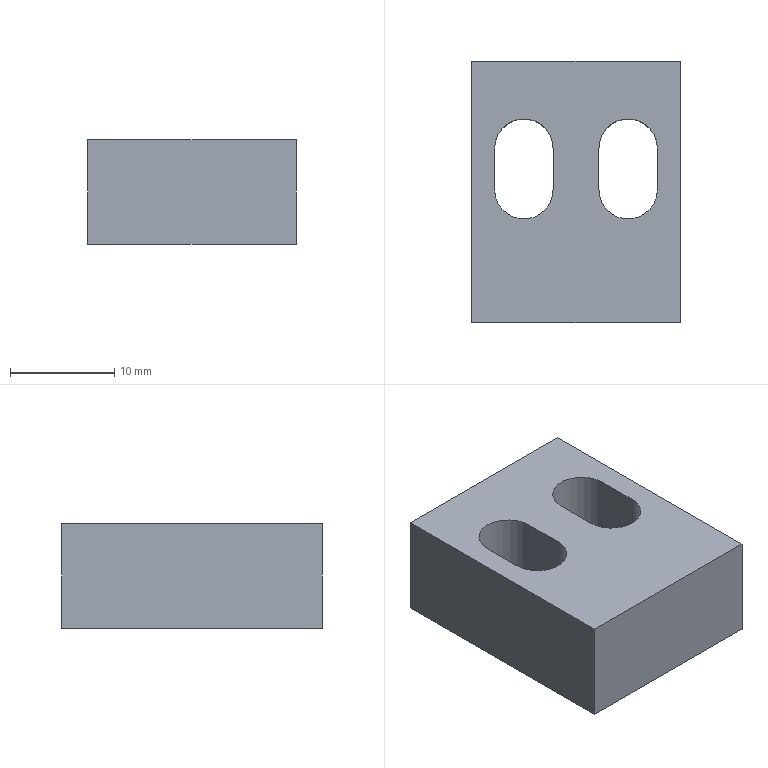Part | 1 solid | 14 faces | box 20 x 25 x 10 mm | volume 4059 mm3 | plane 10 | cylinder 4 | commonest cylinder face diameters 5.6 x4
STEP:
#1=CARTESIAN_POINT('',(-7.8,0.2,10.));
#2=VERTEX_POINT('',#1);
#3=CARTESIAN_POINT('',(-2.2,0.2,10.));
#4=VERTEX_POINT('',#3);
#5=CARTESIAN_POINT('',(-5.,0.2,10.));
#6=DIRECTION('',(0.,0.,1.));
#7=DIRECTION('',(1.,0.,0.));
#8=AXIS2_PLACEMENT_3D('',#5,#6,#7);
#9=CIRCLE('',#8,2.8);
#10=EDGE_CURVE('',#2,#4,#9,.T.);
#11=ORIENTED_EDGE('',*,*,#10,.F.);
#12=CARTESIAN_POINT('',(-7.8,4.2,10.));
#13=VERTEX_POINT('',#12);
#14=CARTESIAN_POINT('',(-7.8,0.2,10.));
#15=DIRECTION('',(0.,-1.,0.));
#16=VECTOR('',#15,1000.);
#17=LINE('',#14,#16);
#18=EDGE_CURVE('',#13,#2,#17,.T.);
#19=ORIENTED_EDGE('',*,*,#18,.F.);
#20=CARTESIAN_POINT('',(-2.2,4.2,10.));
#21=VERTEX_POINT('',#20);
#22=CARTESIAN_POINT('',(-5.,4.2,10.));
#23=DIRECTION('',(0.,0.,1.));
#24=DIRECTION('',(1.,0.,0.));
#25=AXIS2_PLACEMENT_3D('',#22,#23,#24);
#26=CIRCLE('',#25,2.8);
#27=EDGE_CURVE('',#21,#13,#26,.T.);
#28=ORIENTED_EDGE('',*,*,#27,.F.);
#29=CARTESIAN_POINT('',(-2.2,0.2,10.));
#30=DIRECTION('',(0.,1.,0.));
#31=VECTOR('',#30,1000.);
#32=LINE('',#29,#31);
#33=EDGE_CURVE('',#4,#21,#32,.T.);
#34=ORIENTED_EDGE('',*,*,#33,.F.);
#35=EDGE_LOOP('',(#11,#19,#28,#34));
#36=FACE_BOUND('',#35,.T.);
#37=CARTESIAN_POINT('',(10.,-12.5,10.));
#38=VERTEX_POINT('',#37);
#39=CARTESIAN_POINT('',(10.,12.5,10.));
#40=VERTEX_POINT('',#39);
#41=CARTESIAN_POINT('',(10.,-12.5,10.));
#42=DIRECTION('',(0.,1.,0.));
#43=VECTOR('',#42,1000.);
#44=LINE('',#41,#43);
#45=EDGE_CURVE('',#38,#40,#44,.T.);
#46=ORIENTED_EDGE('',*,*,#45,.T.);
#47=CARTESIAN_POINT('',(-10.,12.5,10.));
#48=VERTEX_POINT('',#47);
#49=CARTESIAN_POINT('',(-10.,12.5,10.));
#50=DIRECTION('',(-1.,0.,0.));
#51=VECTOR('',#50,1000.);
#52=LINE('',#49,#51);
#53=EDGE_CURVE('',#40,#48,#52,.T.);
#54=ORIENTED_EDGE('',*,*,#53,.T.);
#55=CARTESIAN_POINT('',(-10.,-12.5,10.));
#56=VERTEX_POINT('',#55);
#57=CARTESIAN_POINT('',(-10.,-12.5,10.));
#58=DIRECTION('',(0.,-1.,0.));
#59=VECTOR('',#58,1000.);
#60=LINE('',#57,#59);
#61=EDGE_CURVE('',#48,#56,#60,.T.);
#62=ORIENTED_EDGE('',*,*,#61,.T.);
#63=CARTESIAN_POINT('',(-10.,-12.5,10.));
#64=DIRECTION('',(1.,0.,0.));
#65=VECTOR('',#64,1000.);
#66=LINE('',#63,#65);
#67=EDGE_CURVE('',#56,#38,#66,.T.);
#68=ORIENTED_EDGE('',*,*,#67,.T.);
#69=EDGE_LOOP('',(#46,#54,#62,#68));
#70=FACE_OUTER_BOUND('',#69,.T.);
#71=CARTESIAN_POINT('',(2.2,0.2,10.));
#72=VERTEX_POINT('',#71);
#73=CARTESIAN_POINT('',(7.8,0.2,10.));
#74=VERTEX_POINT('',#73);
#75=CARTESIAN_POINT('',(5.,0.2,10.));
#76=DIRECTION('',(0.,0.,1.));
#77=DIRECTION('',(-1.,0.,0.));
#78=AXIS2_PLACEMENT_3D('',#75,#76,#77);
#79=CIRCLE('',#78,2.8);
#80=EDGE_CURVE('',#72,#74,#79,.T.);
#81=ORIENTED_EDGE('',*,*,#80,.F.);
#82=CARTESIAN_POINT('',(2.2,4.2,10.));
#83=VERTEX_POINT('',#82);
#84=CARTESIAN_POINT('',(2.2,0.2,10.));
#85=DIRECTION('',(0.,-1.,0.));
#86=VECTOR('',#85,1000.);
#87=LINE('',#84,#86);
#88=EDGE_CURVE('',#83,#72,#87,.T.);
#89=ORIENTED_EDGE('',*,*,#88,.F.);
#90=CARTESIAN_POINT('',(7.8,4.2,10.));
#91=VERTEX_POINT('',#90);
#92=CARTESIAN_POINT('',(5.,4.2,10.));
#93=DIRECTION('',(0.,0.,1.));
#94=DIRECTION('',(-1.,0.,0.));
#95=AXIS2_PLACEMENT_3D('',#92,#93,#94);
#96=CIRCLE('',#95,2.8);
#97=EDGE_CURVE('',#91,#83,#96,.T.);
#98=ORIENTED_EDGE('',*,*,#97,.F.);
#99=CARTESIAN_POINT('',(7.8,0.2,10.));
#100=DIRECTION('',(0.,1.,0.));
#101=VECTOR('',#100,1000.);
#102=LINE('',#99,#101);
#103=EDGE_CURVE('',#74,#91,#102,.T.);
#104=ORIENTED_EDGE('',*,*,#103,.F.);
#105=EDGE_LOOP('',(#81,#89,#98,#104));
#106=FACE_BOUND('',#105,.T.);
#107=CARTESIAN_POINT('',(0.,0.,10.));
#108=DIRECTION('',(0.,0.,-1.));
#109=DIRECTION('',(-1.,0.,0.));
#110=AXIS2_PLACEMENT_3D('',#107,#108,#109);
#111=PLANE('',#110);
#112=ADVANCED_FACE('',(#36,#70,#106),#111,.F.);
#113=CARTESIAN_POINT('',(10.,-12.5,0.));
#114=VERTEX_POINT('',#113);
#115=CARTESIAN_POINT('',(10.,12.5,0.));
#116=VERTEX_POINT('',#115);
#117=CARTESIAN_POINT('',(10.,-12.5,0.));
#118=DIRECTION('',(0.,1.,0.));
#119=VECTOR('',#118,1000.);
#120=LINE('',#117,#119);
#121=EDGE_CURVE('',#114,#116,#120,.T.);
#122=ORIENTED_EDGE('',*,*,#121,.F.);
#123=CARTESIAN_POINT('',(-10.,-12.5,0.));
#124=VERTEX_POINT('',#123);
#125=CARTESIAN_POINT('',(-10.,-12.5,0.));
#126=DIRECTION('',(1.,0.,0.));
#127=VECTOR('',#126,1000.);
#128=LINE('',#125,#127);
#129=EDGE_CURVE('',#124,#114,#128,.T.);
#130=ORIENTED_EDGE('',*,*,#129,.F.);
#131=CARTESIAN_POINT('',(-10.,12.5,0.));
#132=VERTEX_POINT('',#131);
#133=CARTESIAN_POINT('',(-10.,-12.5,0.));
#134=DIRECTION('',(0.,-1.,0.));
#135=VECTOR('',#134,1000.);
#136=LINE('',#133,#135);
#137=EDGE_CURVE('',#132,#124,#136,.T.);
#138=ORIENTED_EDGE('',*,*,#137,.F.);
#139=CARTESIAN_POINT('',(-10.,12.5,0.));
#140=DIRECTION('',(-1.,0.,0.));
#141=VECTOR('',#140,1000.);
#142=LINE('',#139,#141);
#143=EDGE_CURVE('',#116,#132,#142,.T.);
#144=ORIENTED_EDGE('',*,*,#143,.F.);
#145=EDGE_LOOP('',(#122,#130,#138,#144));
#146=FACE_OUTER_BOUND('',#145,.T.);
#147=CARTESIAN_POINT('',(-7.8,4.2,0.));
#148=VERTEX_POINT('',#147);
#149=CARTESIAN_POINT('',(-7.8,0.2,0.));
#150=VERTEX_POINT('',#149);
#151=CARTESIAN_POINT('',(-7.8,0.2,0.));
#152=DIRECTION('',(0.,-1.,0.));
#153=VECTOR('',#152,1000.);
#154=LINE('',#151,#153);
#155=EDGE_CURVE('',#148,#150,#154,.T.);
#156=ORIENTED_EDGE('',*,*,#155,.T.);
#157=CARTESIAN_POINT('',(-2.2,0.2,0.));
#158=VERTEX_POINT('',#157);
#159=CARTESIAN_POINT('',(-5.,0.2,0.));
#160=DIRECTION('',(0.,0.,1.));
#161=DIRECTION('',(1.,0.,0.));
#162=AXIS2_PLACEMENT_3D('',#159,#160,#161);
#163=CIRCLE('',#162,2.8);
#164=EDGE_CURVE('',#150,#158,#163,.T.);
#165=ORIENTED_EDGE('',*,*,#164,.T.);
#166=CARTESIAN_POINT('',(-2.2,4.2,0.));
#167=VERTEX_POINT('',#166);
#168=CARTESIAN_POINT('',(-2.2,0.2,0.));
#169=DIRECTION('',(0.,1.,0.));
#170=VECTOR('',#169,1000.);
#171=LINE('',#168,#170);
#172=EDGE_CURVE('',#158,#167,#171,.T.);
#173=ORIENTED_EDGE('',*,*,#172,.T.);
#174=CARTESIAN_POINT('',(-5.,4.2,0.));
#175=DIRECTION('',(0.,0.,1.));
#176=DIRECTION('',(1.,0.,0.));
#177=AXIS2_PLACEMENT_3D('',#174,#175,#176);
#178=CIRCLE('',#177,2.8);
#179=EDGE_CURVE('',#167,#148,#178,.T.);
#180=ORIENTED_EDGE('',*,*,#179,.T.);
#181=EDGE_LOOP('',(#156,#165,#173,#180));
#182=FACE_BOUND('',#181,.T.);
#183=CARTESIAN_POINT('',(2.2,4.2,0.));
#184=VERTEX_POINT('',#183);
#185=CARTESIAN_POINT('',(2.2,0.2,0.));
#186=VERTEX_POINT('',#185);
#187=CARTESIAN_POINT('',(2.2,0.2,0.));
#188=DIRECTION('',(0.,-1.,0.));
#189=VECTOR('',#188,1000.);
#190=LINE('',#187,#189);
#191=EDGE_CURVE('',#184,#186,#190,.T.);
#192=ORIENTED_EDGE('',*,*,#191,.T.);
#193=CARTESIAN_POINT('',(7.8,0.2,0.));
#194=VERTEX_POINT('',#193);
#195=CARTESIAN_POINT('',(5.,0.2,0.));
#196=DIRECTION('',(0.,0.,1.));
#197=DIRECTION('',(-1.,0.,0.));
#198=AXIS2_PLACEMENT_3D('',#195,#196,#197);
#199=CIRCLE('',#198,2.8);
#200=EDGE_CURVE('',#186,#194,#199,.T.);
#201=ORIENTED_EDGE('',*,*,#200,.T.);
#202=CARTESIAN_POINT('',(7.8,4.2,0.));
#203=VERTEX_POINT('',#202);
#204=CARTESIAN_POINT('',(7.8,0.2,0.));
#205=DIRECTION('',(0.,1.,0.));
#206=VECTOR('',#205,1000.);
#207=LINE('',#204,#206);
#208=EDGE_CURVE('',#194,#203,#207,.T.);
#209=ORIENTED_EDGE('',*,*,#208,.T.);
#210=CARTESIAN_POINT('',(5.,4.2,0.));
#211=DIRECTION('',(0.,0.,1.));
#212=DIRECTION('',(-1.,0.,0.));
#213=AXIS2_PLACEMENT_3D('',#210,#211,#212);
#214=CIRCLE('',#213,2.8);
#215=EDGE_CURVE('',#203,#184,#214,.T.);
#216=ORIENTED_EDGE('',*,*,#215,.T.);
#217=EDGE_LOOP('',(#192,#201,#209,#216));
#218=FACE_BOUND('',#217,.T.);
#219=CARTESIAN_POINT('',(0.,0.,0.));
#220=DIRECTION('',(0.,0.,-1.));
#221=DIRECTION('',(-1.,0.,0.));
#222=AXIS2_PLACEMENT_3D('',#219,#220,#221);
#223=PLANE('',#222);
#224=ADVANCED_FACE('',(#146,#182,#218),#223,.T.);
#225=ORIENTED_EDGE('',*,*,#121,.T.);
#226=CARTESIAN_POINT('',(10.,12.5,10.));
#227=DIRECTION('',(0.,0.,-1.));
#228=VECTOR('',#227,1000.);
#229=LINE('',#226,#228);
#230=EDGE_CURVE('',#40,#116,#229,.T.);
#231=ORIENTED_EDGE('',*,*,#230,.F.);
#232=ORIENTED_EDGE('',*,*,#45,.F.);
#233=CARTESIAN_POINT('',(10.,-12.5,10.));
#234=DIRECTION('',(0.,0.,-1.));
#235=VECTOR('',#234,1000.);
#236=LINE('',#233,#235);
#237=EDGE_CURVE('',#38,#114,#236,.T.);
#238=ORIENTED_EDGE('',*,*,#237,.T.);
#239=EDGE_LOOP('',(#225,#231,#232,#238));
#240=FACE_OUTER_BOUND('',#239,.T.);
#241=CARTESIAN_POINT('',(10.,-12.5,10.));
#242=DIRECTION('',(-1.,0.,0.));
#243=DIRECTION('',(0.,0.,1.));
#244=AXIS2_PLACEMENT_3D('',#241,#242,#243);
#245=PLANE('',#244);
#246=ADVANCED_FACE('',(#240),#245,.F.);
#247=ORIENTED_EDGE('',*,*,#143,.T.);
#248=CARTESIAN_POINT('',(-10.,12.5,10.));
#249=DIRECTION('',(0.,0.,-1.));
#250=VECTOR('',#249,1000.);
#251=LINE('',#248,#250);
#252=EDGE_CURVE('',#48,#132,#251,.T.);
#253=ORIENTED_EDGE('',*,*,#252,.F.);
#254=ORIENTED_EDGE('',*,*,#53,.F.);
#255=ORIENTED_EDGE('',*,*,#230,.T.);
#256=EDGE_LOOP('',(#247,#253,#254,#255));
#257=FACE_OUTER_BOUND('',#256,.T.);
#258=CARTESIAN_POINT('',(-10.,12.5,10.));
#259=DIRECTION('',(0.,-1.,0.));
#260=DIRECTION('',(0.,0.,-1.));
#261=AXIS2_PLACEMENT_3D('',#258,#259,#260);
#262=PLANE('',#261);
#263=ADVANCED_FACE('',(#257),#262,.F.);
#264=ORIENTED_EDGE('',*,*,#137,.T.);
#265=CARTESIAN_POINT('',(-10.,-12.5,10.));
#266=DIRECTION('',(0.,0.,-1.));
#267=VECTOR('',#266,1000.);
#268=LINE('',#265,#267);
#269=EDGE_CURVE('',#56,#124,#268,.T.);
#270=ORIENTED_EDGE('',*,*,#269,.F.);
#271=ORIENTED_EDGE('',*,*,#61,.F.);
#272=ORIENTED_EDGE('',*,*,#252,.T.);
#273=EDGE_LOOP('',(#264,#270,#271,#272));
#274=FACE_OUTER_BOUND('',#273,.T.);
#275=CARTESIAN_POINT('',(-10.,-12.5,10.));
#276=DIRECTION('',(1.,0.,0.));
#277=DIRECTION('',(0.,0.,-1.));
#278=AXIS2_PLACEMENT_3D('',#275,#276,#277);
#279=PLANE('',#278);
#280=ADVANCED_FACE('',(#274),#279,.F.);
#281=ORIENTED_EDGE('',*,*,#129,.T.);
#282=ORIENTED_EDGE('',*,*,#237,.F.);
#283=ORIENTED_EDGE('',*,*,#67,.F.);
#284=ORIENTED_EDGE('',*,*,#269,.T.);
#285=EDGE_LOOP('',(#281,#282,#283,#284));
#286=FACE_OUTER_BOUND('',#285,.T.);
#287=CARTESIAN_POINT('',(-10.,-12.5,10.));
#288=DIRECTION('',(0.,1.,0.));
#289=DIRECTION('',(0.,0.,1.));
#290=AXIS2_PLACEMENT_3D('',#287,#288,#289);
#291=PLANE('',#290);
#292=ADVANCED_FACE('',(#286),#291,.F.);
#293=ORIENTED_EDGE('',*,*,#164,.F.);
#294=CARTESIAN_POINT('',(-7.8,0.2,10.));
#295=DIRECTION('',(0.,0.,-1.));
#296=VECTOR('',#295,1000.);
#297=LINE('',#294,#296);
#298=EDGE_CURVE('',#2,#150,#297,.T.);
#299=ORIENTED_EDGE('',*,*,#298,.F.);
#300=ORIENTED_EDGE('',*,*,#10,.T.);
#301=CARTESIAN_POINT('',(-2.2,0.2,10.));
#302=DIRECTION('',(0.,0.,-1.));
#303=VECTOR('',#302,1000.);
#304=LINE('',#301,#303);
#305=EDGE_CURVE('',#4,#158,#304,.T.);
#306=ORIENTED_EDGE('',*,*,#305,.T.);
#307=EDGE_LOOP('',(#293,#299,#300,#306));
#308=FACE_OUTER_BOUND('',#307,.T.);
#309=CARTESIAN_POINT('',(-5.,0.2,10.));
#310=DIRECTION('',(0.,0.,-1.));
#311=DIRECTION('',(-1.,0.,0.));
#312=AXIS2_PLACEMENT_3D('',#309,#310,#311);
#313=CYLINDRICAL_SURFACE('',#312,2.8);
#314=ADVANCED_FACE('',(#308),#313,.F.);
#315=ORIENTED_EDGE('',*,*,#172,.F.);
#316=ORIENTED_EDGE('',*,*,#305,.F.);
#317=ORIENTED_EDGE('',*,*,#33,.T.);
#318=CARTESIAN_POINT('',(-2.2,4.2,10.));
#319=DIRECTION('',(0.,0.,-1.));
#320=VECTOR('',#319,1000.);
#321=LINE('',#318,#320);
#322=EDGE_CURVE('',#21,#167,#321,.T.);
#323=ORIENTED_EDGE('',*,*,#322,.T.);
#324=EDGE_LOOP('',(#315,#316,#317,#323));
#325=FACE_OUTER_BOUND('',#324,.T.);
#326=CARTESIAN_POINT('',(-2.2,0.2,10.));
#327=DIRECTION('',(-1.,0.,0.));
#328=DIRECTION('',(0.,0.,1.));
#329=AXIS2_PLACEMENT_3D('',#326,#327,#328);
#330=PLANE('',#329);
#331=ADVANCED_FACE('',(#325),#330,.T.);
#332=ORIENTED_EDGE('',*,*,#179,.F.);
#333=ORIENTED_EDGE('',*,*,#322,.F.);
#334=ORIENTED_EDGE('',*,*,#27,.T.);
#335=CARTESIAN_POINT('',(-7.8,4.2,10.));
#336=DIRECTION('',(0.,0.,-1.));
#337=VECTOR('',#336,1000.);
#338=LINE('',#335,#337);
#339=EDGE_CURVE('',#13,#148,#338,.T.);
#340=ORIENTED_EDGE('',*,*,#339,.T.);
#341=EDGE_LOOP('',(#332,#333,#334,#340));
#342=FACE_OUTER_BOUND('',#341,.T.);
#343=CARTESIAN_POINT('',(-5.,4.2,10.));
#344=DIRECTION('',(0.,0.,-1.));
#345=DIRECTION('',(-1.,0.,0.));
#346=AXIS2_PLACEMENT_3D('',#343,#344,#345);
#347=CYLINDRICAL_SURFACE('',#346,2.8);
#348=ADVANCED_FACE('',(#342),#347,.F.);
#349=ORIENTED_EDGE('',*,*,#155,.F.);
#350=ORIENTED_EDGE('',*,*,#339,.F.);
#351=ORIENTED_EDGE('',*,*,#18,.T.);
#352=ORIENTED_EDGE('',*,*,#298,.T.);
#353=EDGE_LOOP('',(#349,#350,#351,#352));
#354=FACE_OUTER_BOUND('',#353,.T.);
#355=CARTESIAN_POINT('',(-7.8,0.2,10.));
#356=DIRECTION('',(1.,0.,0.));
#357=DIRECTION('',(0.,0.,-1.));
#358=AXIS2_PLACEMENT_3D('',#355,#356,#357);
#359=PLANE('',#358);
#360=ADVANCED_FACE('',(#354),#359,.T.);
#361=ORIENTED_EDGE('',*,*,#200,.F.);
#362=CARTESIAN_POINT('',(2.2,0.2,10.));
#363=DIRECTION('',(0.,0.,-1.));
#364=VECTOR('',#363,1000.);
#365=LINE('',#362,#364);
#366=EDGE_CURVE('',#72,#186,#365,.T.);
#367=ORIENTED_EDGE('',*,*,#366,.F.);
#368=ORIENTED_EDGE('',*,*,#80,.T.);
#369=CARTESIAN_POINT('',(7.8,0.2,10.));
#370=DIRECTION('',(0.,0.,-1.));
#371=VECTOR('',#370,1000.);
#372=LINE('',#369,#371);
#373=EDGE_CURVE('',#74,#194,#372,.T.);
#374=ORIENTED_EDGE('',*,*,#373,.T.);
#375=EDGE_LOOP('',(#361,#367,#368,#374));
#376=FACE_OUTER_BOUND('',#375,.T.);
#377=CARTESIAN_POINT('',(5.,0.2,10.));
#378=DIRECTION('',(0.,0.,-1.));
#379=DIRECTION('',(-1.,0.,0.));
#380=AXIS2_PLACEMENT_3D('',#377,#378,#379);
#381=CYLINDRICAL_SURFACE('',#380,2.8);
#382=ADVANCED_FACE('',(#376),#381,.F.);
#383=ORIENTED_EDGE('',*,*,#208,.F.);
#384=ORIENTED_EDGE('',*,*,#373,.F.);
#385=ORIENTED_EDGE('',*,*,#103,.T.);
#386=CARTESIAN_POINT('',(7.8,4.2,10.));
#387=DIRECTION('',(0.,0.,-1.));
#388=VECTOR('',#387,1000.);
#389=LINE('',#386,#388);
#390=EDGE_CURVE('',#91,#203,#389,.T.);
#391=ORIENTED_EDGE('',*,*,#390,.T.);
#392=EDGE_LOOP('',(#383,#384,#385,#391));
#393=FACE_OUTER_BOUND('',#392,.T.);
#394=CARTESIAN_POINT('',(7.8,0.2,10.));
#395=DIRECTION('',(-1.,0.,0.));
#396=DIRECTION('',(0.,-1.,0.));
#397=AXIS2_PLACEMENT_3D('',#394,#395,#396);
#398=PLANE('',#397);
#399=ADVANCED_FACE('',(#393),#398,.T.);
#400=ORIENTED_EDGE('',*,*,#215,.F.);
#401=ORIENTED_EDGE('',*,*,#390,.F.);
#402=ORIENTED_EDGE('',*,*,#97,.T.);
#403=CARTESIAN_POINT('',(2.2,4.2,10.));
#404=DIRECTION('',(0.,0.,-1.));
#405=VECTOR('',#404,1000.);
#406=LINE('',#403,#405);
#407=EDGE_CURVE('',#83,#184,#406,.T.);
#408=ORIENTED_EDGE('',*,*,#407,.T.);
#409=EDGE_LOOP('',(#400,#401,#402,#408));
#410=FACE_OUTER_BOUND('',#409,.T.);
#411=CARTESIAN_POINT('',(5.,4.2,10.));
#412=DIRECTION('',(0.,0.,-1.));
#413=DIRECTION('',(-1.,0.,0.));
#414=AXIS2_PLACEMENT_3D('',#411,#412,#413);
#415=CYLINDRICAL_SURFACE('',#414,2.8);
#416=ADVANCED_FACE('',(#410),#415,.F.);
#417=ORIENTED_EDGE('',*,*,#191,.F.);
#418=ORIENTED_EDGE('',*,*,#407,.F.);
#419=ORIENTED_EDGE('',*,*,#88,.T.);
#420=ORIENTED_EDGE('',*,*,#366,.T.);
#421=EDGE_LOOP('',(#417,#418,#419,#420));
#422=FACE_OUTER_BOUND('',#421,.T.);
#423=CARTESIAN_POINT('',(2.2,0.2,10.));
#424=DIRECTION('',(1.,0.,0.));
#425=DIRECTION('',(0.,1.,0.));
#426=AXIS2_PLACEMENT_3D('',#423,#424,#425);
#427=PLANE('',#426);
#428=ADVANCED_FACE('',(#422),#427,.T.);
#429=CLOSED_SHELL('',(#112,#224,#246,#263,#280,#292,#314,#331,#348,#360,#382,#399,#416,#428));
#430=MANIFOLD_SOLID_BREP('',#429);
#431=CARTESIAN_POINT('',(0.,0.,0.));
#432=DIRECTION('',(0.,0.,1.));
#433=DIRECTION('',(1.,0.,0.));
#434=AXIS2_PLACEMENT_3D('',#431,#432,#433);
#435=(LENGTH_UNIT()NAMED_UNIT(*)SI_UNIT(.MILLI.,.METRE.));
#436=UNCERTAINTY_MEASURE_WITH_UNIT(LENGTH_MEASURE(0.00001),#435,'','');
#437=(NAMED_UNIT(*)PLANE_ANGLE_UNIT()SI_UNIT($,.RADIAN.));
#438=(NAMED_UNIT(*)SI_UNIT($,.STERADIAN.)SOLID_ANGLE_UNIT());
#439=(GEOMETRIC_REPRESENTATION_CONTEXT(3)GLOBAL_UNCERTAINTY_ASSIGNED_CONTEXT((#436))GLOBAL_UNIT_ASSIGNED_CONTEXT((#435,#437,#438))REPRESENTATION_CONTEXT('',''));
#440=ADVANCED_BREP_SHAPE_REPRESENTATION('',(#430,#434),#439);